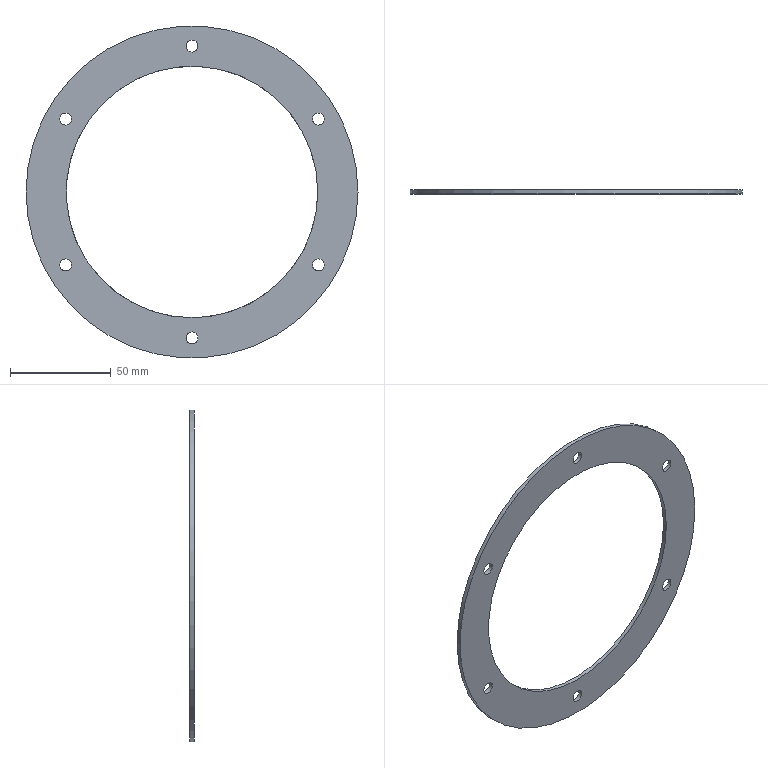Part | NX | features DATUM_CSYS 12, SKETCH 11, HOLE PACKAGE 9, SIMPLE HOLE 9, EXTRACT_DATUM_AXIS 6, EXTRACT_FACE 6, Instance Feature 5, EXTRUDE 4, BLEND 2, DELETE FACE 1, OFFSET_REGION 1, Pattern Feature 1, SWP104 1 | 1 solid | 10 faces | box 165 x 2 x 165 mm | volume 17882 mm3 | cylinder 8 | plane 2 | commonest cylinder face diameters 6 x6 125 x1 165 x1
STEP:
#1=CARTESIAN_POINT('',(82.5,-9.6,0.));
#2=VERTEX_POINT('',#1);
#3=CARTESIAN_POINT('',(0.,-9.6,0.));
#4=DIRECTION('',(0.,-1.,0.));
#5=DIRECTION('',(1.,0.,0.));
#6=AXIS2_PLACEMENT_3D('',#3,#4,#5);
#7=CIRCLE('',#6,82.5);
#8=EDGE_CURVE('',#2,#2,#7,.T.);
#9=ORIENTED_EDGE('',*,*,#8,.F.);
#10=EDGE_LOOP('',(#9));
#11=FACE_BOUND('',#10,.T.);
#12=CARTESIAN_POINT('',(-82.5,-7.6,0.));
#13=VERTEX_POINT('',#12);
#14=CARTESIAN_POINT('',(0.,-7.6,0.));
#15=DIRECTION('',(0.,1.,0.));
#16=DIRECTION('',(-1.,0.,0.));
#17=AXIS2_PLACEMENT_3D('',#14,#15,#16);
#18=CIRCLE('',#17,82.5);
#19=EDGE_CURVE('',#13,#13,#18,.F.);
#20=ORIENTED_EDGE('',*,*,#19,.T.);
#21=EDGE_LOOP('',(#20));
#22=FACE_BOUND('',#21,.T.);
#23=CARTESIAN_POINT('',(0.,0.,0.));
#24=DIRECTION('',(0.,-1.,0.));
#25=DIRECTION('',(0.,0.,-1.));
#26=AXIS2_PLACEMENT_3D('',#23,#24,#25);
#27=CYLINDRICAL_SURFACE('',#26,82.5);
#28=ADVANCED_FACE('',(#11,#22),#27,.T.);
#29=CARTESIAN_POINT('',(0.,-9.6,75.5));
#30=VERTEX_POINT('',#29);
#31=CARTESIAN_POINT('',(0.,-9.6,72.5));
#32=DIRECTION('',(0.,1.,0.));
#33=DIRECTION('',(0.,0.,1.));
#34=AXIS2_PLACEMENT_3D('',#31,#32,#33);
#35=CIRCLE('',#34,3.);
#36=EDGE_CURVE('',#30,#30,#35,.T.);
#37=ORIENTED_EDGE('',*,*,#36,.F.);
#38=EDGE_LOOP('',(#37));
#39=FACE_BOUND('',#38,.T.);
#40=CARTESIAN_POINT('',(-3.,-7.6,72.5));
#41=VERTEX_POINT('',#40);
#42=CARTESIAN_POINT('',(0.,-7.6,72.5));
#43=DIRECTION('',(0.,1.,0.));
#44=DIRECTION('',(-1.,0.,0.));
#45=AXIS2_PLACEMENT_3D('',#42,#43,#44);
#46=CIRCLE('',#45,3.);
#47=EDGE_CURVE('',#41,#41,#46,.F.);
#48=ORIENTED_EDGE('',*,*,#47,.F.);
#49=EDGE_LOOP('',(#48));
#50=FACE_BOUND('',#49,.T.);
#51=CARTESIAN_POINT('',(0.,-9.6,72.5));
#52=DIRECTION('',(0.,1.,0.));
#53=DIRECTION('',(0.,0.,1.));
#54=AXIS2_PLACEMENT_3D('',#51,#52,#53);
#55=CYLINDRICAL_SURFACE('',#54,3.);
#56=ADVANCED_FACE('',(#39,#50),#55,.F.);
#57=CARTESIAN_POINT('',(62.787,-9.6,39.25));
#58=VERTEX_POINT('',#57);
#59=CARTESIAN_POINT('',(62.787,-9.6,36.25));
#60=DIRECTION('',(0.,1.,0.));
#61=DIRECTION('',(0.,0.,1.));
#62=AXIS2_PLACEMENT_3D('',#59,#60,#61);
#63=CIRCLE('',#62,3.);
#64=EDGE_CURVE('',#58,#58,#63,.T.);
#65=ORIENTED_EDGE('',*,*,#64,.F.);
#66=EDGE_LOOP('',(#65));
#67=FACE_BOUND('',#66,.T.);
#68=CARTESIAN_POINT('',(59.787,-7.6,36.25));
#69=VERTEX_POINT('',#68);
#70=CARTESIAN_POINT('',(62.787,-7.6,36.25));
#71=DIRECTION('',(0.,1.,0.));
#72=DIRECTION('',(-1.,0.,0.));
#73=AXIS2_PLACEMENT_3D('',#70,#71,#72);
#74=CIRCLE('',#73,3.);
#75=EDGE_CURVE('',#69,#69,#74,.F.);
#76=ORIENTED_EDGE('',*,*,#75,.F.);
#77=EDGE_LOOP('',(#76));
#78=FACE_BOUND('',#77,.T.);
#79=CARTESIAN_POINT('',(62.787,-9.6,36.25));
#80=DIRECTION('',(0.,1.,0.));
#81=DIRECTION('',(0.,0.,1.));
#82=AXIS2_PLACEMENT_3D('',#79,#80,#81);
#83=CYLINDRICAL_SURFACE('',#82,3.);
#84=ADVANCED_FACE('',(#67,#78),#83,.F.);
#85=CARTESIAN_POINT('',(62.787,-9.6,-33.25));
#86=VERTEX_POINT('',#85);
#87=CARTESIAN_POINT('',(62.787,-9.6,-36.25));
#88=DIRECTION('',(0.,1.,0.));
#89=DIRECTION('',(0.,0.,1.));
#90=AXIS2_PLACEMENT_3D('',#87,#88,#89);
#91=CIRCLE('',#90,3.);
#92=EDGE_CURVE('',#86,#86,#91,.T.);
#93=ORIENTED_EDGE('',*,*,#92,.F.);
#94=EDGE_LOOP('',(#93));
#95=FACE_BOUND('',#94,.T.);
#96=CARTESIAN_POINT('',(59.787,-7.6,-36.25));
#97=VERTEX_POINT('',#96);
#98=CARTESIAN_POINT('',(62.787,-7.6,-36.25));
#99=DIRECTION('',(0.,1.,0.));
#100=DIRECTION('',(-1.,0.,0.));
#101=AXIS2_PLACEMENT_3D('',#98,#99,#100);
#102=CIRCLE('',#101,3.);
#103=EDGE_CURVE('',#97,#97,#102,.F.);
#104=ORIENTED_EDGE('',*,*,#103,.F.);
#105=EDGE_LOOP('',(#104));
#106=FACE_BOUND('',#105,.T.);
#107=CARTESIAN_POINT('',(62.787,-9.6,-36.25));
#108=DIRECTION('',(0.,1.,0.));
#109=DIRECTION('',(0.,0.,1.));
#110=AXIS2_PLACEMENT_3D('',#107,#108,#109);
#111=CYLINDRICAL_SURFACE('',#110,3.);
#112=ADVANCED_FACE('',(#95,#106),#111,.F.);
#113=CARTESIAN_POINT('',(0.,-9.6,-69.5));
#114=VERTEX_POINT('',#113);
#115=CARTESIAN_POINT('',(0.,-9.6,-72.5));
#116=DIRECTION('',(0.,1.,0.));
#117=DIRECTION('',(0.,0.,1.));
#118=AXIS2_PLACEMENT_3D('',#115,#116,#117);
#119=CIRCLE('',#118,3.);
#120=EDGE_CURVE('',#114,#114,#119,.T.);
#121=ORIENTED_EDGE('',*,*,#120,.F.);
#122=EDGE_LOOP('',(#121));
#123=FACE_BOUND('',#122,.T.);
#124=CARTESIAN_POINT('',(-3.,-7.6,-72.5));
#125=VERTEX_POINT('',#124);
#126=CARTESIAN_POINT('',(0.,-7.6,-72.5));
#127=DIRECTION('',(0.,1.,0.));
#128=DIRECTION('',(-1.,0.,0.));
#129=AXIS2_PLACEMENT_3D('',#126,#127,#128);
#130=CIRCLE('',#129,3.);
#131=EDGE_CURVE('',#125,#125,#130,.F.);
#132=ORIENTED_EDGE('',*,*,#131,.F.);
#133=EDGE_LOOP('',(#132));
#134=FACE_BOUND('',#133,.T.);
#135=CARTESIAN_POINT('',(0.,-9.6,-72.5));
#136=DIRECTION('',(0.,1.,0.));
#137=DIRECTION('',(0.,0.,1.));
#138=AXIS2_PLACEMENT_3D('',#135,#136,#137);
#139=CYLINDRICAL_SURFACE('',#138,3.);
#140=ADVANCED_FACE('',(#123,#134),#139,.F.);
#141=CARTESIAN_POINT('',(-62.787,-9.6,-33.25));
#142=VERTEX_POINT('',#141);
#143=CARTESIAN_POINT('',(-62.787,-9.6,-36.25));
#144=DIRECTION('',(0.,1.,0.));
#145=DIRECTION('',(0.,0.,1.));
#146=AXIS2_PLACEMENT_3D('',#143,#144,#145);
#147=CIRCLE('',#146,3.);
#148=EDGE_CURVE('',#142,#142,#147,.T.);
#149=ORIENTED_EDGE('',*,*,#148,.F.);
#150=EDGE_LOOP('',(#149));
#151=FACE_BOUND('',#150,.T.);
#152=CARTESIAN_POINT('',(-65.787,-7.6,-36.25));
#153=VERTEX_POINT('',#152);
#154=CARTESIAN_POINT('',(-62.787,-7.6,-36.25));
#155=DIRECTION('',(0.,1.,0.));
#156=DIRECTION('',(-1.,0.,0.));
#157=AXIS2_PLACEMENT_3D('',#154,#155,#156);
#158=CIRCLE('',#157,3.);
#159=EDGE_CURVE('',#153,#153,#158,.F.);
#160=ORIENTED_EDGE('',*,*,#159,.F.);
#161=EDGE_LOOP('',(#160));
#162=FACE_BOUND('',#161,.T.);
#163=CARTESIAN_POINT('',(-62.787,-9.6,-36.25));
#164=DIRECTION('',(0.,1.,0.));
#165=DIRECTION('',(0.,0.,1.));
#166=AXIS2_PLACEMENT_3D('',#163,#164,#165);
#167=CYLINDRICAL_SURFACE('',#166,3.);
#168=ADVANCED_FACE('',(#151,#162),#167,.F.);
#169=CARTESIAN_POINT('',(-62.787,-9.6,39.25));
#170=VERTEX_POINT('',#169);
#171=CARTESIAN_POINT('',(-62.787,-9.6,36.25));
#172=DIRECTION('',(0.,1.,0.));
#173=DIRECTION('',(0.,0.,1.));
#174=AXIS2_PLACEMENT_3D('',#171,#172,#173);
#175=CIRCLE('',#174,3.);
#176=EDGE_CURVE('',#170,#170,#175,.T.);
#177=ORIENTED_EDGE('',*,*,#176,.F.);
#178=EDGE_LOOP('',(#177));
#179=FACE_BOUND('',#178,.T.);
#180=CARTESIAN_POINT('',(-65.787,-7.6,36.25));
#181=VERTEX_POINT('',#180);
#182=CARTESIAN_POINT('',(-62.787,-7.6,36.25));
#183=DIRECTION('',(0.,1.,0.));
#184=DIRECTION('',(-1.,0.,0.));
#185=AXIS2_PLACEMENT_3D('',#182,#183,#184);
#186=CIRCLE('',#185,3.);
#187=EDGE_CURVE('',#181,#181,#186,.F.);
#188=ORIENTED_EDGE('',*,*,#187,.F.);
#189=EDGE_LOOP('',(#188));
#190=FACE_BOUND('',#189,.T.);
#191=CARTESIAN_POINT('',(-62.787,-9.6,36.25));
#192=DIRECTION('',(0.,1.,0.));
#193=DIRECTION('',(0.,0.,1.));
#194=AXIS2_PLACEMENT_3D('',#191,#192,#193);
#195=CYLINDRICAL_SURFACE('',#194,3.);
#196=ADVANCED_FACE('',(#179,#190),#195,.F.);
#197=CARTESIAN_POINT('',(0.,-9.6,-62.5));
#198=VERTEX_POINT('',#197);
#199=CARTESIAN_POINT('',(0.,-9.6,0.));
#200=DIRECTION('',(0.,-1.,0.));
#201=DIRECTION('',(0.,0.,-1.));
#202=AXIS2_PLACEMENT_3D('',#199,#200,#201);
#203=CIRCLE('',#202,62.5);
#204=EDGE_CURVE('',#198,#198,#203,.T.);
#205=ORIENTED_EDGE('',*,*,#204,.F.);
#206=EDGE_LOOP('',(#205));
#207=FACE_BOUND('',#206,.T.);
#208=ORIENTED_EDGE('',*,*,#176,.T.);
#209=EDGE_LOOP('',(#208));
#210=FACE_BOUND('',#209,.T.);
#211=ORIENTED_EDGE('',*,*,#148,.T.);
#212=EDGE_LOOP('',(#211));
#213=FACE_BOUND('',#212,.T.);
#214=ORIENTED_EDGE('',*,*,#120,.T.);
#215=EDGE_LOOP('',(#214));
#216=FACE_BOUND('',#215,.T.);
#217=ORIENTED_EDGE('',*,*,#92,.T.);
#218=EDGE_LOOP('',(#217));
#219=FACE_BOUND('',#218,.T.);
#220=ORIENTED_EDGE('',*,*,#64,.T.);
#221=EDGE_LOOP('',(#220));
#222=FACE_BOUND('',#221,.T.);
#223=ORIENTED_EDGE('',*,*,#36,.T.);
#224=EDGE_LOOP('',(#223));
#225=FACE_BOUND('',#224,.T.);
#226=ORIENTED_EDGE('',*,*,#8,.T.);
#227=EDGE_LOOP('',(#226));
#228=FACE_BOUND('',#227,.T.);
#229=CARTESIAN_POINT('',(0.,-9.6,0.));
#230=DIRECTION('',(0.,-1.,0.));
#231=DIRECTION('',(0.,0.,-1.));
#232=AXIS2_PLACEMENT_3D('',#229,#230,#231);
#233=PLANE('',#232);
#234=ADVANCED_FACE('',(#207,#210,#213,#216,#219,#222,#225,#228),#233,.T.);
#235=CARTESIAN_POINT('',(62.5,-7.6,0.));
#236=VERTEX_POINT('',#235);
#237=CARTESIAN_POINT('',(0.,-7.6,0.));
#238=DIRECTION('',(0.,1.,0.));
#239=DIRECTION('',(1.,0.,0.));
#240=AXIS2_PLACEMENT_3D('',#237,#238,#239);
#241=CIRCLE('',#240,62.5);
#242=EDGE_CURVE('',#236,#236,#241,.T.);
#243=ORIENTED_EDGE('',*,*,#242,.F.);
#244=EDGE_LOOP('',(#243));
#245=FACE_BOUND('',#244,.T.);
#246=ORIENTED_EDGE('',*,*,#19,.F.);
#247=EDGE_LOOP('',(#246));
#248=FACE_BOUND('',#247,.T.);
#249=ORIENTED_EDGE('',*,*,#187,.T.);
#250=EDGE_LOOP('',(#249));
#251=FACE_BOUND('',#250,.T.);
#252=ORIENTED_EDGE('',*,*,#159,.T.);
#253=EDGE_LOOP('',(#252));
#254=FACE_BOUND('',#253,.T.);
#255=ORIENTED_EDGE('',*,*,#131,.T.);
#256=EDGE_LOOP('',(#255));
#257=FACE_BOUND('',#256,.T.);
#258=ORIENTED_EDGE('',*,*,#103,.T.);
#259=EDGE_LOOP('',(#258));
#260=FACE_BOUND('',#259,.T.);
#261=ORIENTED_EDGE('',*,*,#75,.T.);
#262=EDGE_LOOP('',(#261));
#263=FACE_BOUND('',#262,.T.);
#264=ORIENTED_EDGE('',*,*,#47,.T.);
#265=EDGE_LOOP('',(#264));
#266=FACE_BOUND('',#265,.T.);
#267=CARTESIAN_POINT('',(-98.,-7.6,125.));
#268=DIRECTION('',(0.,1.,0.));
#269=DIRECTION('',(-1.,0.,0.));
#270=AXIS2_PLACEMENT_3D('',#267,#268,#269);
#271=PLANE('',#270);
#272=ADVANCED_FACE('',(#245,#248,#251,#254,#257,#260,#263,#266),#271,.T.);
#273=ORIENTED_EDGE('',*,*,#204,.T.);
#274=EDGE_LOOP('',(#273));
#275=FACE_BOUND('',#274,.T.);
#276=ORIENTED_EDGE('',*,*,#242,.T.);
#277=EDGE_LOOP('',(#276));
#278=FACE_BOUND('',#277,.T.);
#279=CARTESIAN_POINT('',(0.,-32.6,0.));
#280=DIRECTION('',(0.,1.,0.));
#281=DIRECTION('',(0.,0.,1.));
#282=AXIS2_PLACEMENT_3D('',#279,#280,#281);
#283=CYLINDRICAL_SURFACE('',#282,62.5);
#284=ADVANCED_FACE('',(#275,#278),#283,.F.);
#285=CLOSED_SHELL('',(#28,#56,#84,#112,#140,#168,#196,#234,#272,#284));
#286=MANIFOLD_SOLID_BREP('',#285);
#287=(LENGTH_UNIT()NAMED_UNIT(*)SI_UNIT(.MILLI.,.METRE.));
#288=UNCERTAINTY_MEASURE_WITH_UNIT(LENGTH_MEASURE(0.00001),#287,'','');
#289=(NAMED_UNIT(*)PLANE_ANGLE_UNIT()SI_UNIT($,.RADIAN.));
#290=(NAMED_UNIT(*)SI_UNIT($,.STERADIAN.)SOLID_ANGLE_UNIT());
#291=(GEOMETRIC_REPRESENTATION_CONTEXT(3)GLOBAL_UNCERTAINTY_ASSIGNED_CONTEXT((#288))GLOBAL_UNIT_ASSIGNED_CONTEXT((#287,#289,#290))REPRESENTATION_CONTEXT('',''));
#292=ADVANCED_BREP_SHAPE_REPRESENTATION('',(#286),#291);